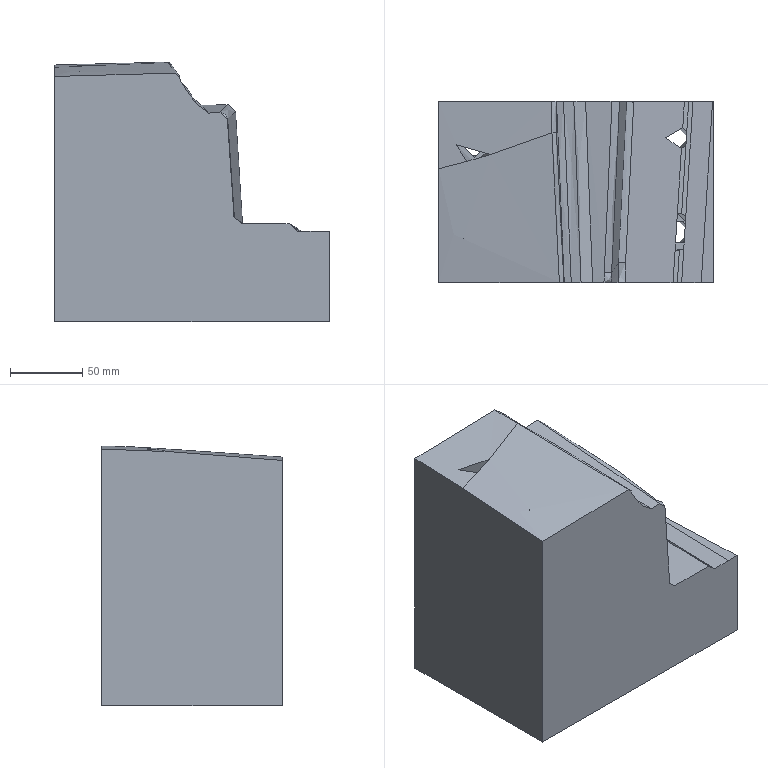Part | NX | features solid 2 | 1 solid | 54 faces | volume 3774392533401089317031637218321530648615864764669773494934723710627048998939276719495456402781796470863327833036057880562458833594179953537503799425329057731505972838400 mm3 | spline 31 | plane 12 | cylinder 11 | commonest cylinder face diameters 16 x2 17 x2 20 x2 25 x2 25.5 x2 25.02 x1